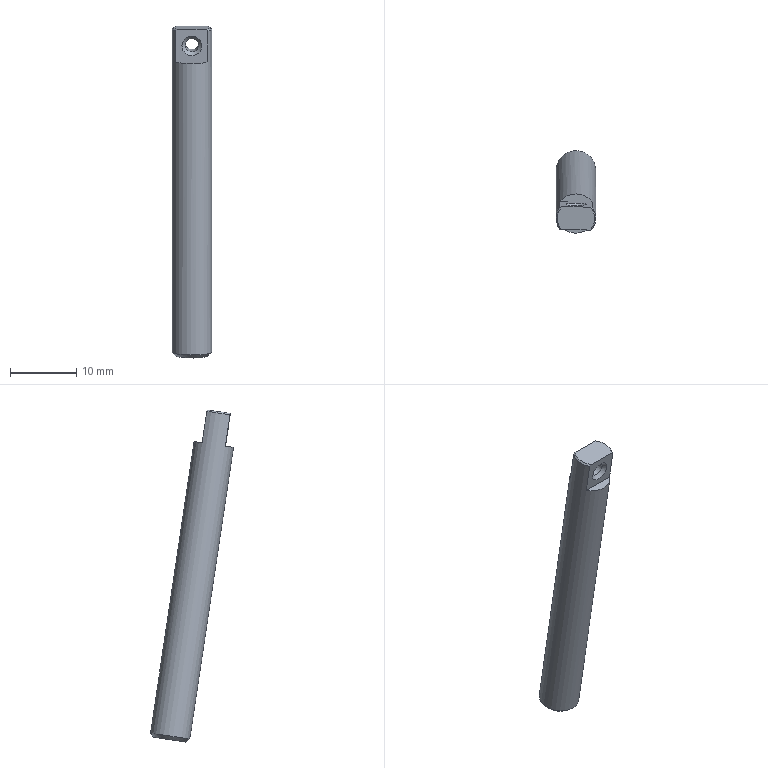Part | NX | features 1 2 | 1 solid | 13 faces | box 6 x 12.52 x 50.075 mm | volume 1355 mm3 | plane 6 | cone 5 | cylinder 2 | commonest cylinder face diameters 2 x1 6 x1
STEP:
#1=CARTESIAN_POINT('',(-77.041,146.086,-986.26));
#2=VERTEX_POINT('',#1);
#3=CARTESIAN_POINT('',(-80.041,146.116,-986.256));
#4=DIRECTION('',(0.,-0.1481,0.989));
#5=DIRECTION('',(0.9999,-0.01016,-0.001522));
#6=AXIS2_PLACEMENT_3D('',#3,#4,#5);
#7=CIRCLE('',#6,3.);
#8=EDGE_CURVE('',#2,#2,#7,.T.);
#9=ORIENTED_EDGE('',*,*,#8,.T.);
#10=EDGE_LOOP('',(#9));
#11=FACE_BOUND('',#10,.T.);
#12=CARTESIAN_POINT('',(-82.496,137.114,-937.796));
#13=VERTEX_POINT('',#12);
#14=CARTESIAN_POINT('',(-82.46,140.575,-937.278));
#15=VERTEX_POINT('',#14);
#16=CARTESIAN_POINT('',(-80.041,138.819,-937.54));
#17=DIRECTION('',(0.,0.1481,-0.989));
#18=DIRECTION('',(0.9999,-0.01016,-0.001522));
#19=AXIS2_PLACEMENT_3D('',#16,#17,#18);
#20=CIRCLE('',#19,3.);
#21=EDGE_CURVE('',#13,#15,#20,.T.);
#22=ORIENTED_EDGE('',*,*,#21,.T.);
#23=CARTESIAN_POINT('',(-82.46,141.286,-942.025));
#24=VERTEX_POINT('',#23);
#25=CARTESIAN_POINT('',(-82.46,144.223,-961.635));
#26=DIRECTION('',(0.,0.1481,-0.989));
#27=VECTOR('',#26,1000.);
#28=LINE('',#25,#27);
#29=EDGE_CURVE('',#15,#24,#28,.T.);
#30=ORIENTED_EDGE('',*,*,#29,.T.);
#31=CARTESIAN_POINT('',(-77.587,141.236,-942.032));
#32=VERTEX_POINT('',#31);
#33=CARTESIAN_POINT('',(-80.041,139.53,-942.288));
#34=DIRECTION('',(0.,0.1481,-0.989));
#35=DIRECTION('',(0.9999,-0.01016,-0.001522));
#36=AXIS2_PLACEMENT_3D('',#33,#34,#35);
#37=CIRCLE('',#36,3.);
#38=EDGE_CURVE('',#24,#32,#37,.T.);
#39=ORIENTED_EDGE('',*,*,#38,.T.);
#40=CARTESIAN_POINT('',(-77.587,140.525,-937.285));
#41=VERTEX_POINT('',#40);
#42=CARTESIAN_POINT('',(-77.587,144.174,-961.642));
#43=DIRECTION('',(0.,-0.1481,0.989));
#44=VECTOR('',#43,1000.);
#45=LINE('',#42,#44);
#46=EDGE_CURVE('',#32,#41,#45,.T.);
#47=ORIENTED_EDGE('',*,*,#46,.T.);
#48=CARTESIAN_POINT('',(-77.623,137.064,-937.803));
#49=VERTEX_POINT('',#48);
#50=CARTESIAN_POINT('',(-80.041,138.819,-937.54));
#51=DIRECTION('',(0.,0.1481,-0.989));
#52=DIRECTION('',(0.9999,-0.01016,-0.001522));
#53=AXIS2_PLACEMENT_3D('',#50,#51,#52);
#54=CIRCLE('',#53,3.);
#55=EDGE_CURVE('',#41,#49,#54,.T.);
#56=ORIENTED_EDGE('',*,*,#55,.T.);
#57=CARTESIAN_POINT('',(-77.623,137.775,-942.55));
#58=VERTEX_POINT('',#57);
#59=CARTESIAN_POINT('',(-77.623,140.712,-962.161));
#60=DIRECTION('',(0.,0.1481,-0.989));
#61=VECTOR('',#60,1000.);
#62=LINE('',#59,#61);
#63=EDGE_CURVE('',#49,#58,#62,.T.);
#64=ORIENTED_EDGE('',*,*,#63,.T.);
#65=CARTESIAN_POINT('',(-82.496,137.825,-942.543));
#66=VERTEX_POINT('',#65);
#67=CARTESIAN_POINT('',(-80.041,139.53,-942.288));
#68=DIRECTION('',(0.,0.1481,-0.989));
#69=DIRECTION('',(0.9999,-0.01016,-0.001522));
#70=AXIS2_PLACEMENT_3D('',#67,#68,#69);
#71=CIRCLE('',#70,3.);
#72=EDGE_CURVE('',#58,#66,#71,.T.);
#73=ORIENTED_EDGE('',*,*,#72,.T.);
#74=CARTESIAN_POINT('',(-82.496,140.762,-962.154));
#75=DIRECTION('',(0.,-0.1481,0.989));
#76=VECTOR('',#75,1000.);
#77=LINE('',#74,#76);
#78=EDGE_CURVE('',#66,#13,#77,.T.);
#79=ORIENTED_EDGE('',*,*,#78,.T.);
#80=EDGE_LOOP('',(#22,#30,#39,#47,#56,#64,#73,#79));
#81=FACE_BOUND('',#80,.T.);
#82=CARTESIAN_POINT('',(-80.041,142.468,-961.898));
#83=DIRECTION('',(0.,0.1481,-0.989));
#84=DIRECTION('',(-0.9999,0.01016,0.001522));
#85=AXIS2_PLACEMENT_3D('',#82,#83,#84);
#86=CYLINDRICAL_SURFACE('',#85,3.);
#87=ADVANCED_FACE('',(#11,#81),#86,.T.);
#88=ORIENTED_EDGE('',*,*,#8,.F.);
#89=EDGE_LOOP('',(#88));
#90=FACE_BOUND('',#89,.T.);
#91=CARTESIAN_POINT('',(-82.5,146.221,-986.787));
#92=VERTEX_POINT('',#91);
#93=CARTESIAN_POINT('',(-80.041,146.196,-986.791));
#94=DIRECTION('',(0.,-0.1481,0.989));
#95=DIRECTION('',(-0.9999,0.01016,0.001522));
#96=AXIS2_PLACEMENT_3D('',#93,#94,#95);
#97=CIRCLE('',#96,2.459);
#98=EDGE_CURVE('',#92,#92,#97,.T.);
#99=ORIENTED_EDGE('',*,*,#98,.T.);
#100=EDGE_LOOP('',(#99));
#101=FACE_BOUND('',#100,.T.);
#102=CARTESIAN_POINT('',(-80.041,146.116,-986.256));
#103=DIRECTION('',(0.,-0.1481,0.989));
#104=DIRECTION('',(0.9999,-0.01016,-0.001522));
#105=AXIS2_PLACEMENT_3D('',#102,#103,#104);
#106=CONICAL_SURFACE('',#105,3.,0.7854);
#107=ADVANCED_FACE('',(#90,#101),#106,.T.);
#108=CARTESIAN_POINT('',(-77.838,140.498,-937.087));
#109=VERTEX_POINT('',#108);
#110=CARTESIAN_POINT('',(-77.874,137.037,-937.605));
#111=VERTEX_POINT('',#110);
#112=CARTESIAN_POINT('',(-80.041,138.79,-937.343));
#113=DIRECTION('',(0.,0.1481,-0.989));
#114=DIRECTION('',(0.9999,-0.01016,-0.001522));
#115=AXIS2_PLACEMENT_3D('',#112,#113,#114);
#116=CIRCLE('',#115,2.8);
#117=EDGE_CURVE('',#109,#111,#116,.T.);
#118=ORIENTED_EDGE('',*,*,#117,.T.);
#119=CARTESIAN_POINT('',(-77.874,137.037,-937.605));
#120=CARTESIAN_POINT('',(-77.789,137.046,-937.67));
#121=CARTESIAN_POINT('',(-77.706,137.055,-937.737));
#122=CARTESIAN_POINT('',(-77.623,137.064,-937.803));
#123=B_SPLINE_CURVE_WITH_KNOTS('',3,(#119,#120,#121,#122),.UNSPECIFIED.,.F.,.F.,(4,4),(0.,1.),.PIECEWISE_BEZIER_KNOTS.);
#124=EDGE_CURVE('',#111,#49,#123,.T.);
#125=ORIENTED_EDGE('',*,*,#124,.T.);
#126=ORIENTED_EDGE('',*,*,#55,.F.);
#127=CARTESIAN_POINT('',(-77.587,140.525,-937.285));
#128=CARTESIAN_POINT('',(-77.67,140.516,-937.218));
#129=CARTESIAN_POINT('',(-77.753,140.507,-937.152));
#130=CARTESIAN_POINT('',(-77.838,140.498,-937.087));
#131=B_SPLINE_CURVE_WITH_KNOTS('',3,(#127,#128,#129,#130),.UNSPECIFIED.,.F.,.F.,(4,4),(0.,1.),.PIECEWISE_BEZIER_KNOTS.);
#132=EDGE_CURVE('',#41,#109,#131,.T.);
#133=ORIENTED_EDGE('',*,*,#132,.T.);
#134=EDGE_LOOP('',(#118,#125,#126,#133));
#135=FACE_BOUND('',#134,.T.);
#136=CARTESIAN_POINT('',(-80.041,138.819,-937.54));
#137=DIRECTION('',(0.,0.1481,-0.989));
#138=DIRECTION('',(-0.9999,0.01016,0.001522));
#139=AXIS2_PLACEMENT_3D('',#136,#137,#138);
#140=CONICAL_SURFACE('',#139,3.,0.7854);
#141=ADVANCED_FACE('',(#135),#140,.T.);
#142=CARTESIAN_POINT('',(-78.523,140.875,-939.558));
#143=VERTEX_POINT('',#142);
#144=CARTESIAN_POINT('',(-80.023,140.891,-939.556));
#145=DIRECTION('',(0.01028,0.9889,0.1481));
#146=DIRECTION('',(0.9999,-0.01016,-0.001522));
#147=AXIS2_PLACEMENT_3D('',#144,#145,#146);
#148=CIRCLE('',#147,1.5);
#149=EDGE_CURVE('',#143,#143,#148,.T.);
#150=ORIENTED_EDGE('',*,*,#149,.T.);
#151=EDGE_LOOP('',(#150));
#152=FACE_BOUND('',#151,.T.);
#153=CARTESIAN_POINT('',(-80.028,140.544,-940.619));
#154=VERTEX_POINT('',#153);
#155=CARTESIAN_POINT('',(-80.028,140.396,-939.63));
#156=DIRECTION('',(0.01028,0.9889,0.1481));
#157=DIRECTION('',(0.,0.1481,-0.989));
#158=AXIS2_PLACEMENT_3D('',#155,#156,#157);
#159=CIRCLE('',#158,1.);
#160=EDGE_CURVE('',#154,#154,#159,.T.);
#161=ORIENTED_EDGE('',*,*,#160,.F.);
#162=EDGE_LOOP('',(#161));
#163=FACE_BOUND('',#162,.T.);
#164=CARTESIAN_POINT('',(-80.023,140.891,-939.556));
#165=DIRECTION('',(0.01028,0.9889,0.1481));
#166=DIRECTION('',(-0.9999,0.01016,0.001522));
#167=AXIS2_PLACEMENT_3D('',#164,#165,#166);
#168=CONICAL_SURFACE('',#167,1.5,0.7854);
#169=ADVANCED_FACE('',(#152,#163),#168,.F.);
#170=CARTESIAN_POINT('',(-81.559,137.445,-940.072));
#171=VERTEX_POINT('',#170);
#172=CARTESIAN_POINT('',(-80.059,137.429,-940.074));
#173=DIRECTION('',(-0.01028,-0.9889,-0.1481));
#174=DIRECTION('',(-0.9999,0.01016,0.001522));
#175=AXIS2_PLACEMENT_3D('',#172,#173,#174);
#176=CIRCLE('',#175,1.5);
#177=EDGE_CURVE('',#171,#171,#176,.T.);
#178=ORIENTED_EDGE('',*,*,#177,.T.);
#179=EDGE_LOOP('',(#178));
#180=FACE_BOUND('',#179,.T.);
#181=CARTESIAN_POINT('',(-80.054,138.072,-940.989));
#182=VERTEX_POINT('',#181);
#183=CARTESIAN_POINT('',(-80.054,137.924,-940.));
#184=DIRECTION('',(-0.01028,-0.9889,-0.1481));
#185=DIRECTION('',(0.,0.1481,-0.989));
#186=AXIS2_PLACEMENT_3D('',#183,#184,#185);
#187=CIRCLE('',#186,1.);
#188=EDGE_CURVE('',#182,#182,#187,.T.);
#189=ORIENTED_EDGE('',*,*,#188,.F.);
#190=EDGE_LOOP('',(#189));
#191=FACE_BOUND('',#190,.T.);
#192=CARTESIAN_POINT('',(-80.059,137.429,-940.074));
#193=DIRECTION('',(-0.01028,-0.9889,-0.1481));
#194=DIRECTION('',(0.9999,-0.01016,-0.001522));
#195=AXIS2_PLACEMENT_3D('',#192,#193,#194);
#196=CONICAL_SURFACE('',#195,1.5,0.7854);
#197=ADVANCED_FACE('',(#180,#191),#196,.F.);
#198=ORIENTED_EDGE('',*,*,#160,.T.);
#199=EDGE_LOOP('',(#198));
#200=FACE_BOUND('',#199,.T.);
#201=ORIENTED_EDGE('',*,*,#188,.T.);
#202=EDGE_LOOP('',(#201));
#203=FACE_BOUND('',#202,.T.);
#204=CARTESIAN_POINT('',(-80.041,139.16,-939.815));
#205=DIRECTION('',(0.01028,0.9889,0.1481));
#206=DIRECTION('',(-0.9999,0.01016,0.001522));
#207=AXIS2_PLACEMENT_3D('',#204,#205,#206);
#208=CYLINDRICAL_SURFACE('',#207,1.);
#209=ADVANCED_FACE('',(#200,#203),#208,.F.);
#210=ORIENTED_EDGE('',*,*,#149,.F.);
#211=EDGE_LOOP('',(#210));
#212=FACE_BOUND('',#211,.T.);
#213=CARTESIAN_POINT('',(-83.023,141.292,-942.024));
#214=DIRECTION('',(0.9999,-0.01016,-0.001522));
#215=VECTOR('',#214,1000.);
#216=LINE('',#213,#215);
#217=EDGE_CURVE('',#24,#32,#216,.T.);
#218=ORIENTED_EDGE('',*,*,#217,.F.);
#219=ORIENTED_EDGE('',*,*,#29,.F.);
#220=CARTESIAN_POINT('',(-82.209,140.543,-937.08));
#221=VERTEX_POINT('',#220);
#222=CARTESIAN_POINT('',(-82.209,140.543,-937.08));
#223=CARTESIAN_POINT('',(-82.293,140.553,-937.145));
#224=CARTESIAN_POINT('',(-82.377,140.564,-937.211));
#225=CARTESIAN_POINT('',(-82.46,140.575,-937.278));
#226=B_SPLINE_CURVE_WITH_KNOTS('',3,(#222,#223,#224,#225),.UNSPECIFIED.,.F.,.F.,(4,4),(0.,1.),.PIECEWISE_BEZIER_KNOTS.);
#227=EDGE_CURVE('',#221,#15,#226,.T.);
#228=ORIENTED_EDGE('',*,*,#227,.F.);
#229=CARTESIAN_POINT('',(-83.023,140.551,-937.079));
#230=DIRECTION('',(-0.9999,0.01016,0.001522));
#231=VECTOR('',#230,1000.);
#232=LINE('',#229,#231);
#233=EDGE_CURVE('',#109,#221,#232,.T.);
#234=ORIENTED_EDGE('',*,*,#233,.F.);
#235=ORIENTED_EDGE('',*,*,#132,.F.);
#236=ORIENTED_EDGE('',*,*,#46,.F.);
#237=EDGE_LOOP('',(#218,#219,#228,#234,#235,#236));
#238=FACE_BOUND('',#237,.T.);
#239=CARTESIAN_POINT('',(-83.023,141.292,-942.024));
#240=DIRECTION('',(-0.01028,-0.9889,-0.1481));
#241=DIRECTION('',(0.9999,-0.01016,-0.001522));
#242=AXIS2_PLACEMENT_3D('',#239,#240,#241);
#243=PLANE('',#242);
#244=ADVANCED_FACE('',(#212,#238),#243,.F.);
#245=CARTESIAN_POINT('',(-82.245,137.081,-937.599));
#246=VERTEX_POINT('',#245);
#247=CARTESIAN_POINT('',(-82.496,137.114,-937.796));
#248=CARTESIAN_POINT('',(-82.413,137.103,-937.729));
#249=CARTESIAN_POINT('',(-82.329,137.092,-937.664));
#250=CARTESIAN_POINT('',(-82.245,137.081,-937.599));
#251=B_SPLINE_CURVE_WITH_KNOTS('',3,(#247,#248,#249,#250),.UNSPECIFIED.,.F.,.F.,(4,4),(0.,1.),.PIECEWISE_BEZIER_KNOTS.);
#252=EDGE_CURVE('',#13,#246,#251,.T.);
#253=ORIENTED_EDGE('',*,*,#252,.T.);
#254=CARTESIAN_POINT('',(-80.041,138.79,-937.343));
#255=DIRECTION('',(0.,0.1481,-0.989));
#256=DIRECTION('',(0.9999,-0.01016,-0.001522));
#257=AXIS2_PLACEMENT_3D('',#254,#255,#256);
#258=CIRCLE('',#257,2.8);
#259=EDGE_CURVE('',#246,#221,#258,.T.);
#260=ORIENTED_EDGE('',*,*,#259,.T.);
#261=ORIENTED_EDGE('',*,*,#227,.T.);
#262=ORIENTED_EDGE('',*,*,#21,.F.);
#263=EDGE_LOOP('',(#253,#260,#261,#262));
#264=FACE_BOUND('',#263,.T.);
#265=CARTESIAN_POINT('',(-80.041,138.819,-937.54));
#266=DIRECTION('',(0.,0.1481,-0.989));
#267=DIRECTION('',(-0.9999,0.01016,0.001522));
#268=AXIS2_PLACEMENT_3D('',#265,#266,#267);
#269=CONICAL_SURFACE('',#268,3.,0.7854);
#270=ADVANCED_FACE('',(#264),#269,.T.);
#271=ORIENTED_EDGE('',*,*,#177,.F.);
#272=EDGE_LOOP('',(#271));
#273=FACE_BOUND('',#272,.T.);
#274=CARTESIAN_POINT('',(-83.059,137.09,-937.597));
#275=DIRECTION('',(0.9999,-0.01016,-0.001522));
#276=VECTOR('',#275,1000.);
#277=LINE('',#274,#276);
#278=EDGE_CURVE('',#246,#111,#277,.T.);
#279=ORIENTED_EDGE('',*,*,#278,.F.);
#280=ORIENTED_EDGE('',*,*,#252,.F.);
#281=ORIENTED_EDGE('',*,*,#78,.F.);
#282=CARTESIAN_POINT('',(-83.059,137.83,-942.542));
#283=DIRECTION('',(-0.9999,0.01016,0.001522));
#284=VECTOR('',#283,1000.);
#285=LINE('',#282,#284);
#286=EDGE_CURVE('',#58,#66,#285,.T.);
#287=ORIENTED_EDGE('',*,*,#286,.F.);
#288=ORIENTED_EDGE('',*,*,#63,.F.);
#289=ORIENTED_EDGE('',*,*,#124,.F.);
#290=EDGE_LOOP('',(#279,#280,#281,#287,#288,#289));
#291=FACE_BOUND('',#290,.T.);
#292=CARTESIAN_POINT('',(-83.059,137.09,-937.597));
#293=DIRECTION('',(0.01028,0.9889,0.1481));
#294=DIRECTION('',(-0.9999,0.01016,0.001522));
#295=AXIS2_PLACEMENT_3D('',#292,#293,#294);
#296=PLANE('',#295);
#297=ADVANCED_FACE('',(#273,#291),#296,.F.);
#298=ORIENTED_EDGE('',*,*,#286,.T.);
#299=ORIENTED_EDGE('',*,*,#72,.F.);
#300=EDGE_LOOP('',(#298,#299));
#301=FACE_BOUND('',#300,.T.);
#302=CARTESIAN_POINT('',(-83.059,137.83,-942.542));
#303=DIRECTION('',(0.,0.1481,-0.989));
#304=DIRECTION('',(-0.9999,0.01016,0.001522));
#305=AXIS2_PLACEMENT_3D('',#302,#303,#304);
#306=PLANE('',#305);
#307=ADVANCED_FACE('',(#301),#306,.F.);
#308=ORIENTED_EDGE('',*,*,#217,.T.);
#309=ORIENTED_EDGE('',*,*,#38,.F.);
#310=EDGE_LOOP('',(#308,#309));
#311=FACE_BOUND('',#310,.T.);
#312=CARTESIAN_POINT('',(-83.005,143.022,-941.765));
#313=DIRECTION('',(0.,0.1481,-0.989));
#314=DIRECTION('',(-0.9999,0.01016,0.001522));
#315=AXIS2_PLACEMENT_3D('',#312,#313,#314);
#316=PLANE('',#315);
#317=ADVANCED_FACE('',(#311),#316,.F.);
#318=ORIENTED_EDGE('',*,*,#98,.F.);
#319=EDGE_LOOP('',(#318));
#320=FACE_BOUND('',#319,.T.);
#321=CARTESIAN_POINT('',(-80.054,144.981,-986.973));
#322=DIRECTION('',(0.,0.1481,-0.989));
#323=DIRECTION('',(-0.9999,0.01016,0.001522));
#324=AXIS2_PLACEMENT_3D('',#321,#322,#323);
#325=PLANE('',#324);
#326=ADVANCED_FACE('',(#320),#325,.T.);
#327=ORIENTED_EDGE('',*,*,#278,.T.);
#328=ORIENTED_EDGE('',*,*,#117,.F.);
#329=ORIENTED_EDGE('',*,*,#233,.T.);
#330=ORIENTED_EDGE('',*,*,#259,.F.);
#331=EDGE_LOOP('',(#327,#328,#329,#330));
#332=FACE_BOUND('',#331,.T.);
#333=CARTESIAN_POINT('',(-80.056,137.405,-937.55));
#334=DIRECTION('',(0.,-0.1481,0.989));
#335=DIRECTION('',(0.9999,-0.01016,-0.001522));
#336=AXIS2_PLACEMENT_3D('',#333,#334,#335);
#337=PLANE('',#336);
#338=ADVANCED_FACE('',(#332),#337,.T.);
#339=CLOSED_SHELL('',(#87,#107,#141,#169,#197,#209,#244,#270,#297,#307,#317,#326,#338));
#340=MANIFOLD_SOLID_BREP('',#339);
#341=(LENGTH_UNIT()NAMED_UNIT(*)SI_UNIT(.MILLI.,.METRE.));
#342=UNCERTAINTY_MEASURE_WITH_UNIT(LENGTH_MEASURE(0.00001),#341,'','');
#343=(NAMED_UNIT(*)PLANE_ANGLE_UNIT()SI_UNIT($,.RADIAN.));
#344=(NAMED_UNIT(*)SI_UNIT($,.STERADIAN.)SOLID_ANGLE_UNIT());
#345=(GEOMETRIC_REPRESENTATION_CONTEXT(3)GLOBAL_UNCERTAINTY_ASSIGNED_CONTEXT((#342))GLOBAL_UNIT_ASSIGNED_CONTEXT((#341,#343,#344))REPRESENTATION_CONTEXT('',''));
#346=ADVANCED_BREP_SHAPE_REPRESENTATION('',(#340),#345);